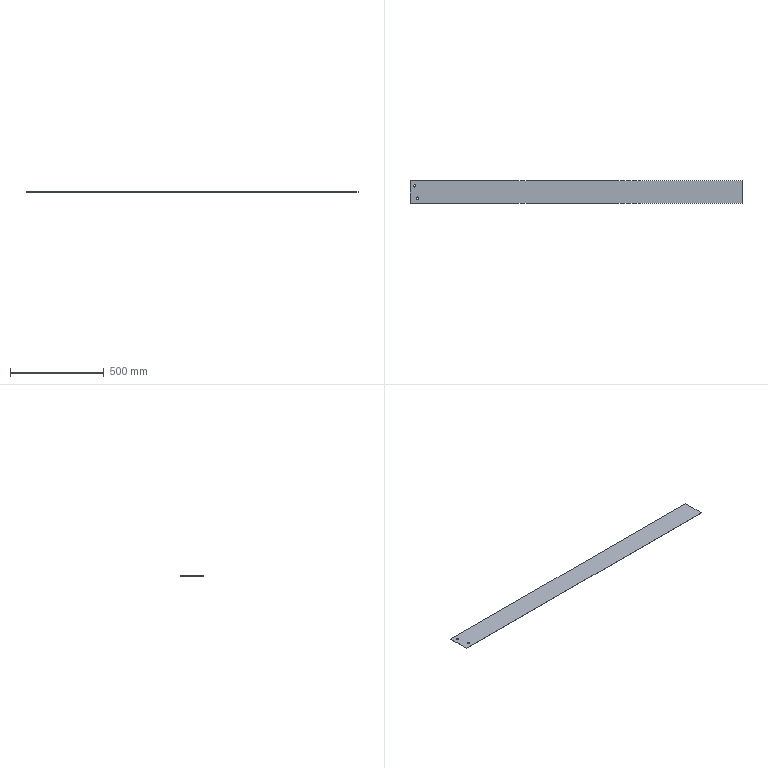Part | SolidWorks | features BaseBody 1 | 1 solid | 10 faces | box 1768 x 120 x 1 mm | volume 211934 mm3 | plane 6 | cylinder 4 | commonest cylinder face diameters 12 x4
STEP:
#1=CARTESIAN_POINT('',(-853.,42.5,1.5));
#2=VERTEX_POINT('',#1);
#3=CARTESIAN_POINT('',(-865.,42.5,1.5));
#4=VERTEX_POINT('',#3);
#5=CARTESIAN_POINT('',(-859.,42.5,1.5));
#6=DIRECTION('',(0.,0.,-1.));
#7=DIRECTION('',(-1.,0.,0.));
#8=AXIS2_PLACEMENT_3D('',#5,#6,#7);
#9=CIRCLE('',#8,6.);
#10=EDGE_CURVE('',#2,#4,#9,.T.);
#11=ORIENTED_EDGE('',*,*,#10,.F.);
#12=CARTESIAN_POINT('',(-853.,42.5,0.5));
#13=VERTEX_POINT('',#12);
#14=CARTESIAN_POINT('',(-853.,42.5,0.5));
#15=DIRECTION('',(0.,0.,-1.));
#16=VECTOR('',#15,1000.);
#17=LINE('',#14,#16);
#18=EDGE_CURVE('',#2,#13,#17,.T.);
#19=ORIENTED_EDGE('',*,*,#18,.T.);
#20=CARTESIAN_POINT('',(-865.,42.5,0.5));
#21=VERTEX_POINT('',#20);
#22=CARTESIAN_POINT('',(-859.,42.5,0.5));
#23=DIRECTION('',(0.,0.,1.));
#24=DIRECTION('',(-1.,0.,0.));
#25=AXIS2_PLACEMENT_3D('',#22,#23,#24);
#26=CIRCLE('',#25,6.);
#27=EDGE_CURVE('',#21,#13,#26,.T.);
#28=ORIENTED_EDGE('',*,*,#27,.F.);
#29=CARTESIAN_POINT('',(-865.,42.5,0.5));
#30=DIRECTION('',(0.,0.,-1.));
#31=VECTOR('',#30,1000.);
#32=LINE('',#29,#31);
#33=EDGE_CURVE('',#4,#21,#32,.T.);
#34=ORIENTED_EDGE('',*,*,#33,.F.);
#35=EDGE_LOOP('',(#11,#19,#28,#34));
#36=FACE_OUTER_BOUND('',#35,.T.);
#37=CARTESIAN_POINT('',(-859.,42.5,0.5));
#38=DIRECTION('',(0.,0.,-1.));
#39=DIRECTION('',(-1.,0.,0.));
#40=AXIS2_PLACEMENT_3D('',#37,#38,#39);
#41=CYLINDRICAL_SURFACE('',#40,6.);
#42=ADVANCED_FACE('',(#36),#41,.F.);
#43=CARTESIAN_POINT('',(-838.,-22.5,1.5));
#44=VERTEX_POINT('',#43);
#45=CARTESIAN_POINT('',(-850.,-22.5,1.5));
#46=VERTEX_POINT('',#45);
#47=CARTESIAN_POINT('',(-844.,-22.5,1.5));
#48=DIRECTION('',(0.,0.,-1.));
#49=DIRECTION('',(-1.,0.,0.));
#50=AXIS2_PLACEMENT_3D('',#47,#48,#49);
#51=CIRCLE('',#50,6.);
#52=EDGE_CURVE('',#44,#46,#51,.T.);
#53=ORIENTED_EDGE('',*,*,#52,.F.);
#54=CARTESIAN_POINT('',(-838.,-22.5,0.5));
#55=VERTEX_POINT('',#54);
#56=CARTESIAN_POINT('',(-838.,-22.5,0.5));
#57=DIRECTION('',(0.,0.,-1.));
#58=VECTOR('',#57,1000.);
#59=LINE('',#56,#58);
#60=EDGE_CURVE('',#44,#55,#59,.T.);
#61=ORIENTED_EDGE('',*,*,#60,.T.);
#62=CARTESIAN_POINT('',(-850.,-22.5,0.5));
#63=VERTEX_POINT('',#62);
#64=CARTESIAN_POINT('',(-844.,-22.5,0.5));
#65=DIRECTION('',(0.,0.,1.));
#66=DIRECTION('',(-1.,0.,0.));
#67=AXIS2_PLACEMENT_3D('',#64,#65,#66);
#68=CIRCLE('',#67,6.);
#69=EDGE_CURVE('',#63,#55,#68,.T.);
#70=ORIENTED_EDGE('',*,*,#69,.F.);
#71=CARTESIAN_POINT('',(-850.,-22.5,0.5));
#72=DIRECTION('',(0.,0.,-1.));
#73=VECTOR('',#72,1000.);
#74=LINE('',#71,#73);
#75=EDGE_CURVE('',#46,#63,#74,.T.);
#76=ORIENTED_EDGE('',*,*,#75,.F.);
#77=EDGE_LOOP('',(#53,#61,#70,#76));
#78=FACE_OUTER_BOUND('',#77,.T.);
#79=CARTESIAN_POINT('',(-844.,-22.5,0.5));
#80=DIRECTION('',(0.,0.,-1.));
#81=DIRECTION('',(-1.,0.,0.));
#82=AXIS2_PLACEMENT_3D('',#79,#80,#81);
#83=CYLINDRICAL_SURFACE('',#82,6.);
#84=ADVANCED_FACE('',(#78),#83,.F.);
#85=CARTESIAN_POINT('',(-859.,42.5,1.5));
#86=DIRECTION('',(0.,0.,-1.));
#87=DIRECTION('',(-1.,0.,0.));
#88=AXIS2_PLACEMENT_3D('',#85,#86,#87);
#89=CIRCLE('',#88,6.);
#90=EDGE_CURVE('',#4,#2,#89,.T.);
#91=ORIENTED_EDGE('',*,*,#90,.T.);
#92=ORIENTED_EDGE('',*,*,#10,.T.);
#93=EDGE_LOOP('',(#91,#92));
#94=FACE_BOUND('',#93,.T.);
#95=CARTESIAN_POINT('',(-844.,-22.5,1.5));
#96=DIRECTION('',(0.,0.,-1.));
#97=DIRECTION('',(-1.,0.,0.));
#98=AXIS2_PLACEMENT_3D('',#95,#96,#97);
#99=CIRCLE('',#98,6.);
#100=EDGE_CURVE('',#46,#44,#99,.T.);
#101=ORIENTED_EDGE('',*,*,#100,.T.);
#102=ORIENTED_EDGE('',*,*,#52,.T.);
#103=EDGE_LOOP('',(#101,#102));
#104=FACE_BOUND('',#103,.T.);
#105=CARTESIAN_POINT('',(884.,-50.,1.5));
#106=VERTEX_POINT('',#105);
#107=CARTESIAN_POINT('',(884.,70.,1.5));
#108=VERTEX_POINT('',#107);
#109=CARTESIAN_POINT('',(884.,834.,1.5));
#110=DIRECTION('',(0.,1.,0.));
#111=VECTOR('',#110,1000.);
#112=LINE('',#109,#111);
#113=EDGE_CURVE('',#106,#108,#112,.T.);
#114=ORIENTED_EDGE('',*,*,#113,.T.);
#115=CARTESIAN_POINT('',(-884.,70.,1.5));
#116=VERTEX_POINT('',#115);
#117=CARTESIAN_POINT('',(0.,70.,1.5));
#118=DIRECTION('',(-1.,0.,0.));
#119=VECTOR('',#118,1000.);
#120=LINE('',#117,#119);
#121=EDGE_CURVE('',#108,#116,#120,.T.);
#122=ORIENTED_EDGE('',*,*,#121,.T.);
#123=CARTESIAN_POINT('',(-884.,-50.,1.5));
#124=VERTEX_POINT('',#123);
#125=CARTESIAN_POINT('',(-884.,834.,1.5));
#126=DIRECTION('',(0.,-1.,0.));
#127=VECTOR('',#126,1000.);
#128=LINE('',#125,#127);
#129=EDGE_CURVE('',#116,#124,#128,.T.);
#130=ORIENTED_EDGE('',*,*,#129,.T.);
#131=CARTESIAN_POINT('',(0.,-50.,1.5));
#132=DIRECTION('',(1.,0.,0.));
#133=VECTOR('',#132,1000.);
#134=LINE('',#131,#133);
#135=EDGE_CURVE('',#124,#106,#134,.T.);
#136=ORIENTED_EDGE('',*,*,#135,.T.);
#137=EDGE_LOOP('',(#114,#122,#130,#136));
#138=FACE_OUTER_BOUND('',#137,.T.);
#139=CARTESIAN_POINT('',(0.,834.,1.5));
#140=DIRECTION('',(0.,0.,1.));
#141=DIRECTION('',(0.,-1.,0.));
#142=AXIS2_PLACEMENT_3D('',#139,#140,#141);
#143=PLANE('',#142);
#144=ADVANCED_FACE('',(#94,#104,#138),#143,.T.);
#145=ORIENTED_EDGE('',*,*,#18,.F.);
#146=ORIENTED_EDGE('',*,*,#90,.F.);
#147=ORIENTED_EDGE('',*,*,#33,.T.);
#148=CARTESIAN_POINT('',(-859.,42.5,0.5));
#149=DIRECTION('',(0.,0.,1.));
#150=DIRECTION('',(-1.,0.,0.));
#151=AXIS2_PLACEMENT_3D('',#148,#149,#150);
#152=CIRCLE('',#151,6.);
#153=EDGE_CURVE('',#13,#21,#152,.T.);
#154=ORIENTED_EDGE('',*,*,#153,.F.);
#155=EDGE_LOOP('',(#145,#146,#147,#154));
#156=FACE_OUTER_BOUND('',#155,.T.);
#157=CARTESIAN_POINT('',(-859.,42.5,0.5));
#158=DIRECTION('',(0.,0.,-1.));
#159=DIRECTION('',(-1.,0.,0.));
#160=AXIS2_PLACEMENT_3D('',#157,#158,#159);
#161=CYLINDRICAL_SURFACE('',#160,6.);
#162=ADVANCED_FACE('',(#156),#161,.F.);
#163=ORIENTED_EDGE('',*,*,#60,.F.);
#164=ORIENTED_EDGE('',*,*,#100,.F.);
#165=ORIENTED_EDGE('',*,*,#75,.T.);
#166=CARTESIAN_POINT('',(-844.,-22.5,0.5));
#167=DIRECTION('',(0.,0.,1.));
#168=DIRECTION('',(-1.,0.,0.));
#169=AXIS2_PLACEMENT_3D('',#166,#167,#168);
#170=CIRCLE('',#169,6.);
#171=EDGE_CURVE('',#55,#63,#170,.T.);
#172=ORIENTED_EDGE('',*,*,#171,.F.);
#173=EDGE_LOOP('',(#163,#164,#165,#172));
#174=FACE_OUTER_BOUND('',#173,.T.);
#175=CARTESIAN_POINT('',(-844.,-22.5,0.5));
#176=DIRECTION('',(0.,0.,-1.));
#177=DIRECTION('',(-1.,0.,0.));
#178=AXIS2_PLACEMENT_3D('',#175,#176,#177);
#179=CYLINDRICAL_SURFACE('',#178,6.);
#180=ADVANCED_FACE('',(#174),#179,.F.);
#181=ORIENTED_EDGE('',*,*,#121,.F.);
#182=CARTESIAN_POINT('',(884.,70.,0.5));
#183=VERTEX_POINT('',#182);
#184=CARTESIAN_POINT('',(884.,70.,1.));
#185=DIRECTION('',(0.,0.,-1.));
#186=VECTOR('',#185,1000.);
#187=LINE('',#184,#186);
#188=EDGE_CURVE('',#108,#183,#187,.T.);
#189=ORIENTED_EDGE('',*,*,#188,.T.);
#190=CARTESIAN_POINT('',(-884.,70.,0.5));
#191=VERTEX_POINT('',#190);
#192=CARTESIAN_POINT('',(0.,70.,0.5));
#193=DIRECTION('',(-1.,0.,0.));
#194=VECTOR('',#193,1000.);
#195=LINE('',#192,#194);
#196=EDGE_CURVE('',#183,#191,#195,.T.);
#197=ORIENTED_EDGE('',*,*,#196,.T.);
#198=CARTESIAN_POINT('',(-884.,70.,1.));
#199=DIRECTION('',(0.,0.,1.));
#200=VECTOR('',#199,1000.);
#201=LINE('',#198,#200);
#202=EDGE_CURVE('',#191,#116,#201,.T.);
#203=ORIENTED_EDGE('',*,*,#202,.T.);
#204=EDGE_LOOP('',(#181,#189,#197,#203));
#205=FACE_OUTER_BOUND('',#204,.T.);
#206=CARTESIAN_POINT('',(0.,70.,1.));
#207=DIRECTION('',(0.,1.,0.));
#208=DIRECTION('',(-1.,0.,0.));
#209=AXIS2_PLACEMENT_3D('',#206,#207,#208);
#210=PLANE('',#209);
#211=ADVANCED_FACE('',(#205),#210,.T.);
#212=ORIENTED_EDGE('',*,*,#113,.F.);
#213=CARTESIAN_POINT('',(884.,-50.,0.5));
#214=VERTEX_POINT('',#213);
#215=CARTESIAN_POINT('',(884.,-50.,1.));
#216=DIRECTION('',(0.,0.,-1.));
#217=VECTOR('',#216,1000.);
#218=LINE('',#215,#217);
#219=EDGE_CURVE('',#106,#214,#218,.T.);
#220=ORIENTED_EDGE('',*,*,#219,.T.);
#221=CARTESIAN_POINT('',(884.,10.,0.5));
#222=DIRECTION('',(0.,1.,0.));
#223=VECTOR('',#222,1000.);
#224=LINE('',#221,#223);
#225=EDGE_CURVE('',#214,#183,#224,.T.);
#226=ORIENTED_EDGE('',*,*,#225,.T.);
#227=ORIENTED_EDGE('',*,*,#188,.F.);
#228=EDGE_LOOP('',(#212,#220,#226,#227));
#229=FACE_OUTER_BOUND('',#228,.T.);
#230=CARTESIAN_POINT('',(884.,10.,1.));
#231=DIRECTION('',(1.,0.,0.));
#232=DIRECTION('',(0.,0.,-1.));
#233=AXIS2_PLACEMENT_3D('',#230,#231,#232);
#234=PLANE('',#233);
#235=ADVANCED_FACE('',(#229),#234,.T.);
#236=ORIENTED_EDGE('',*,*,#135,.F.);
#237=CARTESIAN_POINT('',(-884.,-50.,0.5));
#238=VERTEX_POINT('',#237);
#239=CARTESIAN_POINT('',(-884.,-50.,1.));
#240=DIRECTION('',(0.,0.,-1.));
#241=VECTOR('',#240,1000.);
#242=LINE('',#239,#241);
#243=EDGE_CURVE('',#124,#238,#242,.T.);
#244=ORIENTED_EDGE('',*,*,#243,.T.);
#245=CARTESIAN_POINT('',(0.,-50.,0.5));
#246=DIRECTION('',(1.,0.,0.));
#247=VECTOR('',#246,1000.);
#248=LINE('',#245,#247);
#249=EDGE_CURVE('',#238,#214,#248,.T.);
#250=ORIENTED_EDGE('',*,*,#249,.T.);
#251=ORIENTED_EDGE('',*,*,#219,.F.);
#252=EDGE_LOOP('',(#236,#244,#250,#251));
#253=FACE_OUTER_BOUND('',#252,.T.);
#254=CARTESIAN_POINT('',(0.,-50.,1.));
#255=DIRECTION('',(0.,-1.,0.));
#256=DIRECTION('',(1.,0.,0.));
#257=AXIS2_PLACEMENT_3D('',#254,#255,#256);
#258=PLANE('',#257);
#259=ADVANCED_FACE('',(#253),#258,.T.);
#260=ORIENTED_EDGE('',*,*,#129,.F.);
#261=ORIENTED_EDGE('',*,*,#202,.F.);
#262=CARTESIAN_POINT('',(-884.,10.,0.5));
#263=DIRECTION('',(0.,-1.,0.));
#264=VECTOR('',#263,1000.);
#265=LINE('',#262,#264);
#266=EDGE_CURVE('',#191,#238,#265,.T.);
#267=ORIENTED_EDGE('',*,*,#266,.T.);
#268=ORIENTED_EDGE('',*,*,#243,.F.);
#269=EDGE_LOOP('',(#260,#261,#267,#268));
#270=FACE_OUTER_BOUND('',#269,.T.);
#271=CARTESIAN_POINT('',(-884.,10.,1.));
#272=DIRECTION('',(-1.,0.,0.));
#273=DIRECTION('',(0.,0.,1.));
#274=AXIS2_PLACEMENT_3D('',#271,#272,#273);
#275=PLANE('',#274);
#276=ADVANCED_FACE('',(#270),#275,.T.);
#277=ORIENTED_EDGE('',*,*,#27,.T.);
#278=ORIENTED_EDGE('',*,*,#153,.T.);
#279=EDGE_LOOP('',(#277,#278));
#280=FACE_BOUND('',#279,.T.);
#281=ORIENTED_EDGE('',*,*,#69,.T.);
#282=ORIENTED_EDGE('',*,*,#171,.T.);
#283=EDGE_LOOP('',(#281,#282));
#284=FACE_BOUND('',#283,.T.);
#285=ORIENTED_EDGE('',*,*,#249,.F.);
#286=ORIENTED_EDGE('',*,*,#266,.F.);
#287=ORIENTED_EDGE('',*,*,#196,.F.);
#288=ORIENTED_EDGE('',*,*,#225,.F.);
#289=EDGE_LOOP('',(#285,#286,#287,#288));
#290=FACE_OUTER_BOUND('',#289,.T.);
#291=CARTESIAN_POINT('',(0.,834.,0.5));
#292=DIRECTION('',(0.,0.,-1.));
#293=DIRECTION('',(0.,1.,0.));
#294=AXIS2_PLACEMENT_3D('',#291,#292,#293);
#295=PLANE('',#294);
#296=ADVANCED_FACE('',(#280,#284,#290),#295,.T.);
#297=CLOSED_SHELL('',(#42,#84,#144,#162,#180,#211,#235,#259,#276,#296));
#298=MANIFOLD_SOLID_BREP('',#297);
#299=CARTESIAN_POINT('',(0.,0.,0.));
#300=DIRECTION('',(0.,0.,1.));
#301=DIRECTION('',(1.,0.,0.));
#302=AXIS2_PLACEMENT_3D('',#299,#300,#301);
#303=(LENGTH_UNIT()NAMED_UNIT(*)SI_UNIT(.MILLI.,.METRE.));
#304=UNCERTAINTY_MEASURE_WITH_UNIT(LENGTH_MEASURE(0.00001),#303,'','');
#305=(NAMED_UNIT(*)PLANE_ANGLE_UNIT()SI_UNIT($,.RADIAN.));
#306=(NAMED_UNIT(*)SI_UNIT($,.STERADIAN.)SOLID_ANGLE_UNIT());
#307=(GEOMETRIC_REPRESENTATION_CONTEXT(3)GLOBAL_UNCERTAINTY_ASSIGNED_CONTEXT((#304))GLOBAL_UNIT_ASSIGNED_CONTEXT((#303,#305,#306))REPRESENTATION_CONTEXT('',''));
#308=ADVANCED_BREP_SHAPE_REPRESENTATION('',(#298,#302),#307);